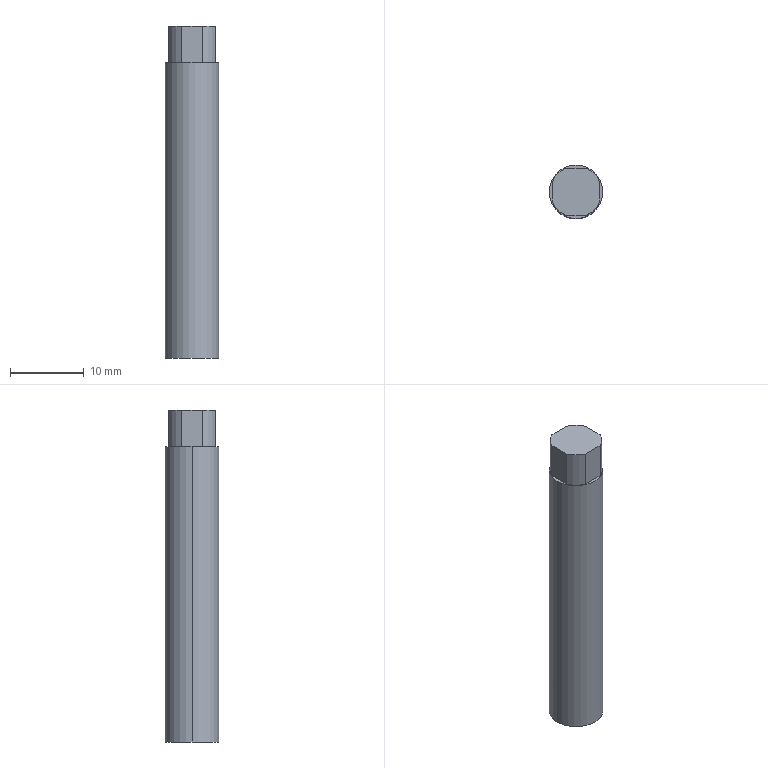Part | NX | 1 solid | 13 faces | box 7.25 x 7.25 x 45 mm | volume 1832 mm3 | plane 7 | cylinder 6 | commonest cylinder face diameters 7 x4 7.25 x2
STEP:
#1=CARTESIAN_POINT('',(3.625,0.,0.));
#2=VERTEX_POINT('',#1);
#3=CARTESIAN_POINT('',(-3.625,0.,0.));
#4=VERTEX_POINT('',#3);
#5=CARTESIAN_POINT('',(0.,0.,0.));
#6=DIRECTION('',(0.,0.,1.));
#7=DIRECTION('',(-1.,0.,0.));
#8=AXIS2_PLACEMENT_3D('',#5,#6,#7);
#9=CIRCLE('',#8,3.625);
#10=EDGE_CURVE('',#2,#4,#9,.T.);
#11=ORIENTED_EDGE('',*,*,#10,.F.);
#12=CARTESIAN_POINT('',(0.,0.,0.));
#13=DIRECTION('',(0.,0.,1.));
#14=DIRECTION('',(-1.,0.,0.));
#15=AXIS2_PLACEMENT_3D('',#12,#13,#14);
#16=CIRCLE('',#15,3.625);
#17=EDGE_CURVE('',#4,#2,#16,.T.);
#18=ORIENTED_EDGE('',*,*,#17,.F.);
#19=EDGE_LOOP('',(#11,#18));
#20=FACE_BOUND('',#19,.T.);
#21=CARTESIAN_POINT('',(0.,0.,0.));
#22=DIRECTION('',(0.,0.,1.));
#23=DIRECTION('',(1.,0.,0.));
#24=AXIS2_PLACEMENT_3D('',#21,#22,#23);
#25=PLANE('',#24);
#26=ADVANCED_FACE('',(#20),#25,.F.);
#27=CARTESIAN_POINT('',(-3.625,0.,40.));
#28=VERTEX_POINT('',#27);
#29=CARTESIAN_POINT('',(3.625,0.,40.));
#30=VERTEX_POINT('',#29);
#31=CARTESIAN_POINT('',(0.,0.,40.));
#32=DIRECTION('',(0.,0.,-1.));
#33=DIRECTION('',(-1.,0.,0.));
#34=AXIS2_PLACEMENT_3D('',#31,#32,#33);
#35=CIRCLE('',#34,3.625);
#36=EDGE_CURVE('',#28,#30,#35,.T.);
#37=ORIENTED_EDGE('',*,*,#36,.T.);
#38=CARTESIAN_POINT('',(3.625,0.,0.));
#39=DIRECTION('',(0.,0.,1.));
#40=VECTOR('',#39,1000.);
#41=LINE('',#38,#40);
#42=EDGE_CURVE('',#2,#30,#41,.T.);
#43=ORIENTED_EDGE('',*,*,#42,.F.);
#44=ORIENTED_EDGE('',*,*,#10,.T.);
#45=CARTESIAN_POINT('',(-3.625,0.,0.));
#46=DIRECTION('',(0.,0.,1.));
#47=VECTOR('',#46,1000.);
#48=LINE('',#45,#47);
#49=EDGE_CURVE('',#4,#28,#48,.T.);
#50=ORIENTED_EDGE('',*,*,#49,.T.);
#51=EDGE_LOOP('',(#37,#43,#44,#50));
#52=FACE_BOUND('',#51,.T.);
#53=CARTESIAN_POINT('',(0.,0.,0.));
#54=DIRECTION('',(0.,0.,1.));
#55=DIRECTION('',(1.,0.,0.));
#56=AXIS2_PLACEMENT_3D('',#53,#54,#55);
#57=CYLINDRICAL_SURFACE('',#56,3.625);
#58=ADVANCED_FACE('',(#52),#57,.T.);
#59=CARTESIAN_POINT('',(-3.2,1.418,45.));
#60=VERTEX_POINT('',#59);
#61=CARTESIAN_POINT('',(-1.418,3.2,45.));
#62=VERTEX_POINT('',#61);
#63=CARTESIAN_POINT('',(0.,0.,45.));
#64=DIRECTION('',(0.,0.,-1.));
#65=DIRECTION('',(-0.9143,0.4051,0.));
#66=AXIS2_PLACEMENT_3D('',#63,#64,#65);
#67=CIRCLE('',#66,3.5);
#68=EDGE_CURVE('',#60,#62,#67,.T.);
#69=ORIENTED_EDGE('',*,*,#68,.T.);
#70=CARTESIAN_POINT('',(-1.418,3.2,40.));
#71=VERTEX_POINT('',#70);
#72=CARTESIAN_POINT('',(-1.418,3.2,40.));
#73=DIRECTION('',(0.,0.,1.));
#74=VECTOR('',#73,1000.);
#75=LINE('',#72,#74);
#76=EDGE_CURVE('',#71,#62,#75,.T.);
#77=ORIENTED_EDGE('',*,*,#76,.F.);
#78=CARTESIAN_POINT('',(-3.2,1.418,40.));
#79=VERTEX_POINT('',#78);
#80=CARTESIAN_POINT('',(0.,0.,40.));
#81=DIRECTION('',(0.,0.,1.));
#82=DIRECTION('',(-0.4051,0.9143,0.));
#83=AXIS2_PLACEMENT_3D('',#80,#81,#82);
#84=CIRCLE('',#83,3.5);
#85=EDGE_CURVE('',#71,#79,#84,.T.);
#86=ORIENTED_EDGE('',*,*,#85,.T.);
#87=CARTESIAN_POINT('',(-3.2,1.418,45.));
#88=DIRECTION('',(0.,0.,-1.));
#89=VECTOR('',#88,1000.);
#90=LINE('',#87,#89);
#91=EDGE_CURVE('',#60,#79,#90,.T.);
#92=ORIENTED_EDGE('',*,*,#91,.F.);
#93=EDGE_LOOP('',(#69,#77,#86,#92));
#94=FACE_BOUND('',#93,.T.);
#95=CARTESIAN_POINT('',(0.,0.,40.));
#96=DIRECTION('',(0.,0.,1.));
#97=DIRECTION('',(0.,-1.,0.));
#98=AXIS2_PLACEMENT_3D('',#95,#96,#97);
#99=CYLINDRICAL_SURFACE('',#98,3.5);
#100=ADVANCED_FACE('',(#94),#99,.T.);
#101=ORIENTED_EDGE('',*,*,#36,.F.);
#102=CARTESIAN_POINT('',(0.,0.,40.));
#103=DIRECTION('',(0.,0.,-1.));
#104=DIRECTION('',(-1.,0.,0.));
#105=AXIS2_PLACEMENT_3D('',#102,#103,#104);
#106=CIRCLE('',#105,3.625);
#107=EDGE_CURVE('',#30,#28,#106,.T.);
#108=ORIENTED_EDGE('',*,*,#107,.F.);
#109=EDGE_LOOP('',(#101,#108));
#110=FACE_BOUND('',#109,.T.);
#111=CARTESIAN_POINT('',(3.2,1.418,40.));
#112=VERTEX_POINT('',#111);
#113=CARTESIAN_POINT('',(1.418,3.2,40.));
#114=VERTEX_POINT('',#113);
#115=CARTESIAN_POINT('',(0.,0.,40.));
#116=DIRECTION('',(0.,0.,1.));
#117=DIRECTION('',(0.9143,0.4051,0.));
#118=AXIS2_PLACEMENT_3D('',#115,#116,#117);
#119=CIRCLE('',#118,3.5);
#120=EDGE_CURVE('',#112,#114,#119,.T.);
#121=ORIENTED_EDGE('',*,*,#120,.F.);
#122=CARTESIAN_POINT('',(3.2,-1.418,40.));
#123=VERTEX_POINT('',#122);
#124=CARTESIAN_POINT('',(3.2,-1.418,40.));
#125=DIRECTION('',(0.,1.,0.));
#126=VECTOR('',#125,1000.);
#127=LINE('',#124,#126);
#128=EDGE_CURVE('',#123,#112,#127,.T.);
#129=ORIENTED_EDGE('',*,*,#128,.F.);
#130=CARTESIAN_POINT('',(1.418,-3.2,40.));
#131=VERTEX_POINT('',#130);
#132=CARTESIAN_POINT('',(0.,0.,40.));
#133=DIRECTION('',(0.,0.,1.));
#134=DIRECTION('',(0.4051,-0.9143,0.));
#135=AXIS2_PLACEMENT_3D('',#132,#133,#134);
#136=CIRCLE('',#135,3.5);
#137=EDGE_CURVE('',#131,#123,#136,.T.);
#138=ORIENTED_EDGE('',*,*,#137,.F.);
#139=CARTESIAN_POINT('',(-1.418,-3.2,40.));
#140=VERTEX_POINT('',#139);
#141=CARTESIAN_POINT('',(-1.418,-3.2,40.));
#142=DIRECTION('',(1.,0.,0.));
#143=VECTOR('',#142,1000.);
#144=LINE('',#141,#143);
#145=EDGE_CURVE('',#140,#131,#144,.T.);
#146=ORIENTED_EDGE('',*,*,#145,.F.);
#147=CARTESIAN_POINT('',(-3.2,-1.418,40.));
#148=VERTEX_POINT('',#147);
#149=CARTESIAN_POINT('',(0.,0.,40.));
#150=DIRECTION('',(0.,0.,1.));
#151=DIRECTION('',(-0.9143,-0.4051,0.));
#152=AXIS2_PLACEMENT_3D('',#149,#150,#151);
#153=CIRCLE('',#152,3.5);
#154=EDGE_CURVE('',#148,#140,#153,.T.);
#155=ORIENTED_EDGE('',*,*,#154,.F.);
#156=CARTESIAN_POINT('',(-3.2,-1.418,40.));
#157=DIRECTION('',(0.,1.,0.));
#158=VECTOR('',#157,1000.);
#159=LINE('',#156,#158);
#160=EDGE_CURVE('',#148,#79,#159,.T.);
#161=ORIENTED_EDGE('',*,*,#160,.T.);
#162=ORIENTED_EDGE('',*,*,#85,.F.);
#163=CARTESIAN_POINT('',(-1.418,3.2,40.));
#164=DIRECTION('',(1.,0.,0.));
#165=VECTOR('',#164,1000.);
#166=LINE('',#163,#165);
#167=EDGE_CURVE('',#71,#114,#166,.T.);
#168=ORIENTED_EDGE('',*,*,#167,.T.);
#169=EDGE_LOOP('',(#121,#129,#138,#146,#155,#161,#162,#168));
#170=FACE_BOUND('',#169,.T.);
#171=CARTESIAN_POINT('',(0.,0.,40.));
#172=DIRECTION('',(0.,0.,1.));
#173=DIRECTION('',(1.,0.,0.));
#174=AXIS2_PLACEMENT_3D('',#171,#172,#173);
#175=PLANE('',#174);
#176=ADVANCED_FACE('',(#110,#170),#175,.T.);
#177=CARTESIAN_POINT('',(1.418,3.2,45.));
#178=VERTEX_POINT('',#177);
#179=CARTESIAN_POINT('',(1.418,3.2,45.));
#180=DIRECTION('',(0.,0.,-1.));
#181=VECTOR('',#180,1000.);
#182=LINE('',#179,#181);
#183=EDGE_CURVE('',#178,#114,#182,.T.);
#184=ORIENTED_EDGE('',*,*,#183,.F.);
#185=CARTESIAN_POINT('',(3.2,1.418,45.));
#186=VERTEX_POINT('',#185);
#187=CARTESIAN_POINT('',(0.,0.,45.));
#188=DIRECTION('',(0.,0.,-1.));
#189=DIRECTION('',(0.4051,0.9143,0.));
#190=AXIS2_PLACEMENT_3D('',#187,#188,#189);
#191=CIRCLE('',#190,3.5);
#192=EDGE_CURVE('',#178,#186,#191,.T.);
#193=ORIENTED_EDGE('',*,*,#192,.T.);
#194=CARTESIAN_POINT('',(3.2,1.418,40.));
#195=DIRECTION('',(0.,0.,1.));
#196=VECTOR('',#195,1000.);
#197=LINE('',#194,#196);
#198=EDGE_CURVE('',#112,#186,#197,.T.);
#199=ORIENTED_EDGE('',*,*,#198,.F.);
#200=ORIENTED_EDGE('',*,*,#120,.T.);
#201=EDGE_LOOP('',(#184,#193,#199,#200));
#202=FACE_BOUND('',#201,.T.);
#203=CARTESIAN_POINT('',(0.,0.,40.));
#204=DIRECTION('',(0.,0.,1.));
#205=DIRECTION('',(0.,-1.,0.));
#206=AXIS2_PLACEMENT_3D('',#203,#204,#205);
#207=CYLINDRICAL_SURFACE('',#206,3.5);
#208=ADVANCED_FACE('',(#202),#207,.T.);
#209=CARTESIAN_POINT('',(1.418,3.2,45.));
#210=DIRECTION('',(-1.,0.,0.));
#211=VECTOR('',#210,1000.);
#212=LINE('',#209,#211);
#213=EDGE_CURVE('',#178,#62,#212,.T.);
#214=ORIENTED_EDGE('',*,*,#213,.F.);
#215=ORIENTED_EDGE('',*,*,#183,.T.);
#216=ORIENTED_EDGE('',*,*,#167,.F.);
#217=ORIENTED_EDGE('',*,*,#76,.T.);
#218=EDGE_LOOP('',(#214,#215,#216,#217));
#219=FACE_BOUND('',#218,.T.);
#220=CARTESIAN_POINT('',(5.724,3.2,45.));
#221=DIRECTION('',(0.,-1.,0.));
#222=DIRECTION('',(0.,0.,-1.));
#223=AXIS2_PLACEMENT_3D('',#220,#221,#222);
#224=PLANE('',#223);
#225=ADVANCED_FACE('',(#219),#224,.F.);
#226=CARTESIAN_POINT('',(1.418,-3.2,45.));
#227=VERTEX_POINT('',#226);
#228=CARTESIAN_POINT('',(-1.418,-3.2,45.));
#229=VERTEX_POINT('',#228);
#230=CARTESIAN_POINT('',(1.418,-3.2,45.));
#231=DIRECTION('',(-1.,0.,0.));
#232=VECTOR('',#231,1000.);
#233=LINE('',#230,#232);
#234=EDGE_CURVE('',#227,#229,#233,.T.);
#235=ORIENTED_EDGE('',*,*,#234,.F.);
#236=CARTESIAN_POINT('',(3.2,-1.418,45.));
#237=VERTEX_POINT('',#236);
#238=CARTESIAN_POINT('',(0.,0.,45.));
#239=DIRECTION('',(0.,0.,-1.));
#240=DIRECTION('',(0.9143,-0.4051,0.));
#241=AXIS2_PLACEMENT_3D('',#238,#239,#240);
#242=CIRCLE('',#241,3.5);
#243=EDGE_CURVE('',#237,#227,#242,.T.);
#244=ORIENTED_EDGE('',*,*,#243,.F.);
#245=CARTESIAN_POINT('',(3.2,1.418,45.));
#246=DIRECTION('',(0.,-1.,0.));
#247=VECTOR('',#246,1000.);
#248=LINE('',#245,#247);
#249=EDGE_CURVE('',#186,#237,#248,.T.);
#250=ORIENTED_EDGE('',*,*,#249,.F.);
#251=ORIENTED_EDGE('',*,*,#192,.F.);
#252=ORIENTED_EDGE('',*,*,#213,.T.);
#253=ORIENTED_EDGE('',*,*,#68,.F.);
#254=CARTESIAN_POINT('',(-3.2,-1.418,45.));
#255=VERTEX_POINT('',#254);
#256=CARTESIAN_POINT('',(-3.2,1.418,45.));
#257=DIRECTION('',(0.,-1.,0.));
#258=VECTOR('',#257,1000.);
#259=LINE('',#256,#258);
#260=EDGE_CURVE('',#60,#255,#259,.T.);
#261=ORIENTED_EDGE('',*,*,#260,.T.);
#262=CARTESIAN_POINT('',(0.,0.,45.));
#263=DIRECTION('',(0.,0.,-1.));
#264=DIRECTION('',(-0.4051,-0.9143,0.));
#265=AXIS2_PLACEMENT_3D('',#262,#263,#264);
#266=CIRCLE('',#265,3.5);
#267=EDGE_CURVE('',#229,#255,#266,.T.);
#268=ORIENTED_EDGE('',*,*,#267,.F.);
#269=EDGE_LOOP('',(#235,#244,#250,#251,#252,#253,#261,#268));
#270=FACE_BOUND('',#269,.T.);
#271=CARTESIAN_POINT('',(0.,0.,45.));
#272=DIRECTION('',(0.,0.,1.));
#273=DIRECTION('',(1.,0.,0.));
#274=AXIS2_PLACEMENT_3D('',#271,#272,#273);
#275=PLANE('',#274);
#276=ADVANCED_FACE('',(#270),#275,.T.);
#277=ORIENTED_EDGE('',*,*,#234,.T.);
#278=CARTESIAN_POINT('',(-1.418,-3.2,45.));
#279=DIRECTION('',(0.,0.,-1.));
#280=VECTOR('',#279,1000.);
#281=LINE('',#278,#280);
#282=EDGE_CURVE('',#229,#140,#281,.T.);
#283=ORIENTED_EDGE('',*,*,#282,.T.);
#284=ORIENTED_EDGE('',*,*,#145,.T.);
#285=CARTESIAN_POINT('',(1.418,-3.2,40.));
#286=DIRECTION('',(0.,0.,1.));
#287=VECTOR('',#286,1000.);
#288=LINE('',#285,#287);
#289=EDGE_CURVE('',#131,#227,#288,.T.);
#290=ORIENTED_EDGE('',*,*,#289,.T.);
#291=EDGE_LOOP('',(#277,#283,#284,#290));
#292=FACE_BOUND('',#291,.T.);
#293=CARTESIAN_POINT('',(5.724,-3.2,40.));
#294=DIRECTION('',(0.,1.,0.));
#295=DIRECTION('',(1.,0.,0.));
#296=AXIS2_PLACEMENT_3D('',#293,#294,#295);
#297=PLANE('',#296);
#298=ADVANCED_FACE('',(#292),#297,.F.);
#299=ORIENTED_EDGE('',*,*,#137,.T.);
#300=CARTESIAN_POINT('',(3.2,-1.418,45.));
#301=DIRECTION('',(0.,0.,-1.));
#302=VECTOR('',#301,1000.);
#303=LINE('',#300,#302);
#304=EDGE_CURVE('',#237,#123,#303,.T.);
#305=ORIENTED_EDGE('',*,*,#304,.F.);
#306=ORIENTED_EDGE('',*,*,#243,.T.);
#307=ORIENTED_EDGE('',*,*,#289,.F.);
#308=EDGE_LOOP('',(#299,#305,#306,#307));
#309=FACE_BOUND('',#308,.T.);
#310=CARTESIAN_POINT('',(0.,0.,40.));
#311=DIRECTION('',(0.,0.,1.));
#312=DIRECTION('',(0.,-1.,0.));
#313=AXIS2_PLACEMENT_3D('',#310,#311,#312);
#314=CYLINDRICAL_SURFACE('',#313,3.5);
#315=ADVANCED_FACE('',(#309),#314,.T.);
#316=ORIENTED_EDGE('',*,*,#249,.T.);
#317=ORIENTED_EDGE('',*,*,#304,.T.);
#318=ORIENTED_EDGE('',*,*,#128,.T.);
#319=ORIENTED_EDGE('',*,*,#198,.T.);
#320=EDGE_LOOP('',(#316,#317,#318,#319));
#321=FACE_BOUND('',#320,.T.);
#322=CARTESIAN_POINT('',(3.2,5.724,40.));
#323=DIRECTION('',(-1.,0.,0.));
#324=DIRECTION('',(0.,0.,1.));
#325=AXIS2_PLACEMENT_3D('',#322,#323,#324);
#326=PLANE('',#325);
#327=ADVANCED_FACE('',(#321),#326,.F.);
#328=ORIENTED_EDGE('',*,*,#282,.F.);
#329=ORIENTED_EDGE('',*,*,#267,.T.);
#330=CARTESIAN_POINT('',(-3.2,-1.418,40.));
#331=DIRECTION('',(0.,0.,1.));
#332=VECTOR('',#331,1000.);
#333=LINE('',#330,#332);
#334=EDGE_CURVE('',#148,#255,#333,.T.);
#335=ORIENTED_EDGE('',*,*,#334,.F.);
#336=ORIENTED_EDGE('',*,*,#154,.T.);
#337=EDGE_LOOP('',(#328,#329,#335,#336));
#338=FACE_BOUND('',#337,.T.);
#339=CARTESIAN_POINT('',(0.,0.,40.));
#340=DIRECTION('',(0.,0.,1.));
#341=DIRECTION('',(0.,-1.,0.));
#342=AXIS2_PLACEMENT_3D('',#339,#340,#341);
#343=CYLINDRICAL_SURFACE('',#342,3.5);
#344=ADVANCED_FACE('',(#338),#343,.T.);
#345=ORIENTED_EDGE('',*,*,#260,.F.);
#346=ORIENTED_EDGE('',*,*,#91,.T.);
#347=ORIENTED_EDGE('',*,*,#160,.F.);
#348=ORIENTED_EDGE('',*,*,#334,.T.);
#349=EDGE_LOOP('',(#345,#346,#347,#348));
#350=FACE_BOUND('',#349,.T.);
#351=CARTESIAN_POINT('',(-3.2,5.724,45.));
#352=DIRECTION('',(1.,0.,0.));
#353=DIRECTION('',(0.,1.,0.));
#354=AXIS2_PLACEMENT_3D('',#351,#352,#353);
#355=PLANE('',#354);
#356=ADVANCED_FACE('',(#350),#355,.F.);
#357=ORIENTED_EDGE('',*,*,#42,.T.);
#358=ORIENTED_EDGE('',*,*,#107,.T.);
#359=ORIENTED_EDGE('',*,*,#49,.F.);
#360=ORIENTED_EDGE('',*,*,#17,.T.);
#361=EDGE_LOOP('',(#357,#358,#359,#360));
#362=FACE_BOUND('',#361,.T.);
#363=CARTESIAN_POINT('',(0.,0.,0.));
#364=DIRECTION('',(0.,0.,1.));
#365=DIRECTION('',(1.,0.,0.));
#366=AXIS2_PLACEMENT_3D('',#363,#364,#365);
#367=CYLINDRICAL_SURFACE('',#366,3.625);
#368=ADVANCED_FACE('',(#362),#367,.T.);
#369=CLOSED_SHELL('',(#26,#58,#100,#176,#208,#225,#276,#298,#315,#327,#344,#356,#368));
#370=MANIFOLD_SOLID_BREP('',#369);
#371=(LENGTH_UNIT()NAMED_UNIT(*)SI_UNIT(.MILLI.,.METRE.));
#372=UNCERTAINTY_MEASURE_WITH_UNIT(LENGTH_MEASURE(0.00001),#371,'','');
#373=(NAMED_UNIT(*)PLANE_ANGLE_UNIT()SI_UNIT($,.RADIAN.));
#374=(NAMED_UNIT(*)SI_UNIT($,.STERADIAN.)SOLID_ANGLE_UNIT());
#375=(GEOMETRIC_REPRESENTATION_CONTEXT(3)GLOBAL_UNCERTAINTY_ASSIGNED_CONTEXT((#372))GLOBAL_UNIT_ASSIGNED_CONTEXT((#371,#373,#374))REPRESENTATION_CONTEXT('',''));
#376=ADVANCED_BREP_SHAPE_REPRESENTATION('',(#370),#375);